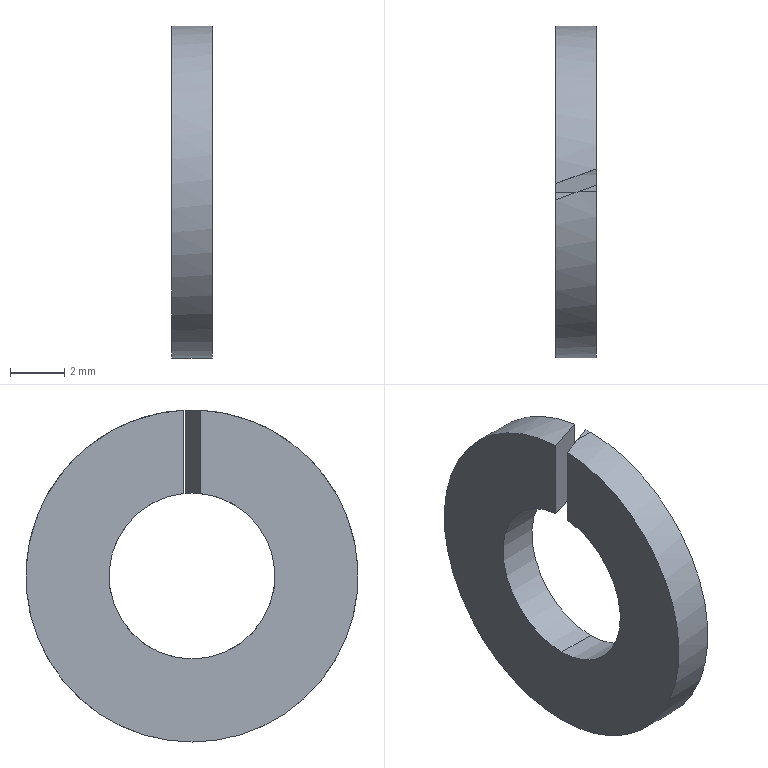Part | STEP file | 0217_302_SLW6 | 1 solid | 10 faces | box 1.5 x 12.2 x 12.2 mm | volume 128.756 mm3 | cylinder 6 | plane 4 | commonest cylinder face diameters 6.1 x3 12.2 x3
STEP:
#1=CARTESIAN_POINT('',(0.,0.,0.));
#2=DIRECTION('',(0.,0.,1.));
#3=DIRECTION('',(1.,0.,0.));
#4=AXIS2_PLACEMENT_3D('',#1,#2,#3);
#5=CARTESIAN_POINT('',(1.5,0.246,6.095));
#6=VERTEX_POINT('',#5);
#7=CARTESIAN_POINT('',(0.8242,0.,6.1));
#8=VERTEX_POINT('',#7);
#9=CARTESIAN_POINT('',(1.5,0.246,6.095));
#10=CARTESIAN_POINT('',(1.275,0.164,6.098));
#11=CARTESIAN_POINT('',(1.05,0.08201,6.1));
#12=CARTESIAN_POINT('',(0.8242,0.,6.1));
#13=(BOUNDED_CURVE()B_SPLINE_CURVE(3,(#9,#10,#11,#12),.UNSPECIFIED.,.F.,.F.)B_SPLINE_CURVE_WITH_KNOTS((4,4),(1.53,1.571),.PIECEWISE_BEZIER_KNOTS.)CURVE()GEOMETRIC_REPRESENTATION_ITEM()RATIONAL_B_SPLINE_CURVE((1.,0.9999,0.9999,1.))REPRESENTATION_ITEM(''));
#14=CARTESIAN_POINT('',(0.,0.,0.));
#15=DIRECTION('',(1.,0.,0.));
#16=DIRECTION('',(0.,0.,-1.));
#17=AXIS2_PLACEMENT_3D('',#14,#15,#16);
#18=CYLINDRICAL_SURFACE('',#17,6.1);
#19=CARTESIAN_POINT('',(3.101,1.5));
#20=CARTESIAN_POINT('',(3.102,1.49));
#21=CARTESIAN_POINT('',(3.103,1.469));
#22=CARTESIAN_POINT('',(3.105,1.439));
#23=CARTESIAN_POINT('',(3.107,1.408));
#24=CARTESIAN_POINT('',(3.109,1.377));
#25=CARTESIAN_POINT('',(3.11,1.346));
#26=CARTESIAN_POINT('',(3.112,1.316));
#27=CARTESIAN_POINT('',(3.114,1.285));
#28=CARTESIAN_POINT('',(3.116,1.254));
#29=CARTESIAN_POINT('',(3.118,1.224));
#30=CARTESIAN_POINT('',(3.12,1.193));
#31=CARTESIAN_POINT('',(3.121,1.162));
#32=CARTESIAN_POINT('',(3.123,1.131));
#33=CARTESIAN_POINT('',(3.125,1.101));
#34=CARTESIAN_POINT('',(3.127,1.07));
#35=CARTESIAN_POINT('',(3.129,1.039));
#36=CARTESIAN_POINT('',(3.131,1.009));
#37=CARTESIAN_POINT('',(3.132,0.9779));
#38=CARTESIAN_POINT('',(3.134,0.9471));
#39=CARTESIAN_POINT('',(3.136,0.9164));
#40=CARTESIAN_POINT('',(3.138,0.8857));
#41=CARTESIAN_POINT('',(3.14,0.855));
#42=CARTESIAN_POINT('',(3.141,0.8345));
#43=CARTESIAN_POINT('',(3.142,0.8242));
#44=B_SPLINE_CURVE_WITH_KNOTS('',3,(#19,#20,#21,#22,#23,#24,#25,#26,#27,#28,#29,#30,#31,#32,#33,#34,#35,#36,#37,#38,#39,#40,#41,#42,#43),.UNSPECIFIED.,.F.,.F.,(4,1,1,1,1,1,1,1,1,1,1,1,1,1,1,1,1,1,1,1,1,1,4),(1.53,1.532,1.534,1.536,1.538,1.54,1.541,1.543,1.545,1.547,1.549,1.551,1.552,1.554,1.556,1.558,1.56,1.562,1.563,1.565,1.567,1.569,1.571),.QUASI_UNIFORM_KNOTS.);
#45=(GEOMETRIC_REPRESENTATION_CONTEXT(2)PARAMETRIC_REPRESENTATION_CONTEXT()REPRESENTATION_CONTEXT('',''));
#46=DEFINITIONAL_REPRESENTATION('',(#44),#45);
#47=PCURVE('',#18,#46);
#48=CARTESIAN_POINT('',(1.5,0.246,0.));
#49=DIRECTION('',(0.342,-0.9397,0.));
#50=DIRECTION('',(0.9397,0.342,0.));
#51=AXIS2_PLACEMENT_3D('',#48,#49,#50);
#52=PLANE('',#51);
#53=CARTESIAN_POINT('',(0.,6.095));
#54=CARTESIAN_POINT('',(-0.2396,6.098));
#55=CARTESIAN_POINT('',(-0.4793,6.1));
#56=CARTESIAN_POINT('',(-0.7191,6.1));
#57=(BOUNDED_CURVE()B_SPLINE_CURVE(3,(#53,#54,#55,#56),.UNSPECIFIED.,.F.,.F.)B_SPLINE_CURVE_WITH_KNOTS((4,4),(1.53,1.571),.PIECEWISE_BEZIER_KNOTS.)CURVE()GEOMETRIC_REPRESENTATION_ITEM()RATIONAL_B_SPLINE_CURVE((1.,0.9999,0.9999,1.))REPRESENTATION_ITEM(''));
#58=(GEOMETRIC_REPRESENTATION_CONTEXT(2)PARAMETRIC_REPRESENTATION_CONTEXT()REPRESENTATION_CONTEXT('',''));
#59=DEFINITIONAL_REPRESENTATION('',(#57),#58);
#60=PCURVE('',#52,#59);
#61=SURFACE_CURVE('',#13,(#47,#60),.PCURVE_S1.);
#62=EDGE_CURVE('',#6,#8,#61,.T.);
#63=ORIENTED_EDGE('',*,*,#62,.T.);
#64=CARTESIAN_POINT('',(1.5,0.,6.1));
#65=VERTEX_POINT('',#64);
#66=CARTESIAN_POINT('',(0.,0.,6.1));
#67=DIRECTION('',(1.,0.,0.));
#68=VECTOR('',#67,1.);
#69=LINE('',#66,#68);
#70=CARTESIAN_POINT('',(3.142,0.));
#71=DIRECTION('',(0.,1.));
#72=VECTOR('',#71,1.);
#73=LINE('',#70,#72);
#74=(GEOMETRIC_REPRESENTATION_CONTEXT(2)PARAMETRIC_REPRESENTATION_CONTEXT()REPRESENTATION_CONTEXT('',''));
#75=DEFINITIONAL_REPRESENTATION('',(#73),#74);
#76=PCURVE('',#18,#75);
#77=CARTESIAN_POINT('',(0.,0.,0.));
#78=DIRECTION('',(1.,0.,0.));
#79=DIRECTION('',(0.,0.,-1.));
#80=AXIS2_PLACEMENT_3D('',#77,#78,#79);
#81=CYLINDRICAL_SURFACE('',#80,6.1);
#82=CARTESIAN_POINT('',(3.142,0.));
#83=DIRECTION('',(0.,1.));
#84=VECTOR('',#83,1.);
#85=LINE('',#82,#84);
#86=(GEOMETRIC_REPRESENTATION_CONTEXT(2)PARAMETRIC_REPRESENTATION_CONTEXT()REPRESENTATION_CONTEXT('',''));
#87=DEFINITIONAL_REPRESENTATION('',(#85),#86);
#88=PCURVE('',#81,#87);
#89=SURFACE_CURVE('',#69,(#76,#88),.PCURVE_S1.);
#90=EDGE_CURVE('',#8,#65,#89,.T.);
#91=ORIENTED_EDGE('',*,*,#90,.T.);
#92=CARTESIAN_POINT('',(1.5,0.,0.));
#93=DIRECTION('',(-1.,0.,0.));
#94=DIRECTION('',(0.,0.,-1.));
#95=AXIS2_PLACEMENT_3D('',#92,#93,#94);
#96=CIRCLE('',#95,6.1);
#97=CARTESIAN_POINT('',(6.283,1.5));
#98=DIRECTION('',(-1.,0.));
#99=VECTOR('',#98,1.);
#100=LINE('',#97,#99);
#101=(GEOMETRIC_REPRESENTATION_CONTEXT(2)PARAMETRIC_REPRESENTATION_CONTEXT()REPRESENTATION_CONTEXT('',''));
#102=DEFINITIONAL_REPRESENTATION('',(#100),#101);
#103=PCURVE('',#18,#102);
#104=CARTESIAN_POINT('',(1.5,0.,0.));
#105=DIRECTION('',(-1.,0.,0.));
#106=DIRECTION('',(0.,0.,1.));
#107=AXIS2_PLACEMENT_3D('',#104,#105,#106);
#108=PLANE('',#107);
#109=CARTESIAN_POINT('',(0.,0.));
#110=DIRECTION('',(-1.,0.));
#111=AXIS2_PLACEMENT_2D('',#109,#110);
#112=CIRCLE('',#111,6.1);
#113=(GEOMETRIC_REPRESENTATION_CONTEXT(2)PARAMETRIC_REPRESENTATION_CONTEXT()REPRESENTATION_CONTEXT('',''));
#114=DEFINITIONAL_REPRESENTATION('',(#112),#113);
#115=PCURVE('',#108,#114);
#116=SURFACE_CURVE('',#96,(#103,#115),.PCURVE_S1.);
#117=EDGE_CURVE('',#65,#6,#116,.T.);
#118=ORIENTED_EDGE('',*,*,#117,.T.);
#119=EDGE_LOOP('',(#63,#91,#118));
#120=FACE_BOUND('',#119,.T.);
#121=ADVANCED_FACE('',(#120),#18,.T.);
#122=ORIENTED_EDGE('',*,*,#90,.F.);
#123=CARTESIAN_POINT('',(0.,-0.3,6.093));
#124=VERTEX_POINT('',#123);
#125=CARTESIAN_POINT('',(0.8242,0.,6.1));
#126=CARTESIAN_POINT('',(0.5494,-0.1001,6.1));
#127=CARTESIAN_POINT('',(0.2746,-0.2001,6.098));
#128=CARTESIAN_POINT('',(0.,-0.3,6.093));
#129=(BOUNDED_CURVE()B_SPLINE_CURVE(3,(#125,#126,#127,#128),.UNSPECIFIED.,.F.,.F.)B_SPLINE_CURVE_WITH_KNOTS((4,4),(1.571,1.62),.PIECEWISE_BEZIER_KNOTS.)CURVE()GEOMETRIC_REPRESENTATION_ITEM()RATIONAL_B_SPLINE_CURVE((1.,0.9998,0.9998,1.))REPRESENTATION_ITEM(''));
#130=CARTESIAN_POINT('',(3.142,0.8242));
#131=CARTESIAN_POINT('',(3.142,0.8118));
#132=CARTESIAN_POINT('',(3.144,0.7868));
#133=CARTESIAN_POINT('',(3.146,0.7493));
#134=CARTESIAN_POINT('',(3.148,0.7118));
#135=CARTESIAN_POINT('',(3.151,0.6743));
#136=CARTESIAN_POINT('',(3.153,0.6369));
#137=CARTESIAN_POINT('',(3.155,0.5994));
#138=CARTESIAN_POINT('',(3.157,0.5619));
#139=CARTESIAN_POINT('',(3.159,0.5244));
#140=CARTESIAN_POINT('',(3.162,0.4869));
#141=CARTESIAN_POINT('',(3.164,0.4495));
#142=CARTESIAN_POINT('',(3.166,0.412));
#143=CARTESIAN_POINT('',(3.168,0.3745));
#144=CARTESIAN_POINT('',(3.171,0.3371));
#145=CARTESIAN_POINT('',(3.173,0.2996));
#146=CARTESIAN_POINT('',(3.175,0.2621));
#147=CARTESIAN_POINT('',(3.177,0.2247));
#148=CARTESIAN_POINT('',(3.18,0.1872));
#149=CARTESIAN_POINT('',(3.182,0.1498));
#150=CARTESIAN_POINT('',(3.184,0.1123));
#151=CARTESIAN_POINT('',(3.186,0.07487));
#152=CARTESIAN_POINT('',(3.189,0.03743));
#153=CARTESIAN_POINT('',(3.19,0.01248));
#154=CARTESIAN_POINT('',(3.191,0.));
#155=B_SPLINE_CURVE_WITH_KNOTS('',3,(#130,#131,#132,#133,#134,#135,#136,#137,#138,#139,#140,#141,#142,#143,#144,#145,#146,#147,#148,#149,#150,#151,#152,#153,#154),.UNSPECIFIED.,.F.,.F.,(4,1,1,1,1,1,1,1,1,1,1,1,1,1,1,1,1,1,1,1,1,1,4),(1.571,1.573,1.575,1.578,1.58,1.582,1.584,1.586,1.589,1.591,1.593,1.595,1.598,1.6,1.602,1.604,1.607,1.609,1.611,1.613,1.616,1.618,1.62),.QUASI_UNIFORM_KNOTS.);
#156=(GEOMETRIC_REPRESENTATION_CONTEXT(2)PARAMETRIC_REPRESENTATION_CONTEXT()REPRESENTATION_CONTEXT('',''));
#157=DEFINITIONAL_REPRESENTATION('',(#155),#156);
#158=PCURVE('',#81,#157);
#159=CARTESIAN_POINT('',(-0.7191,6.1));
#160=CARTESIAN_POINT('',(-1.012,6.1));
#161=CARTESIAN_POINT('',(-1.304,6.098));
#162=CARTESIAN_POINT('',(-1.596,6.093));
#163=(BOUNDED_CURVE()B_SPLINE_CURVE(3,(#159,#160,#161,#162),.UNSPECIFIED.,.F.,.F.)B_SPLINE_CURVE_WITH_KNOTS((4,4),(1.571,1.62),.PIECEWISE_BEZIER_KNOTS.)CURVE()GEOMETRIC_REPRESENTATION_ITEM()RATIONAL_B_SPLINE_CURVE((1.,0.9998,0.9998,1.))REPRESENTATION_ITEM(''));
#164=(GEOMETRIC_REPRESENTATION_CONTEXT(2)PARAMETRIC_REPRESENTATION_CONTEXT()REPRESENTATION_CONTEXT('',''));
#165=DEFINITIONAL_REPRESENTATION('',(#163),#164);
#166=PCURVE('',#52,#165);
#167=SURFACE_CURVE('',#129,(#158,#166),.PCURVE_S1.);
#168=EDGE_CURVE('',#8,#124,#167,.T.);
#169=ORIENTED_EDGE('',*,*,#168,.T.);
#170=CARTESIAN_POINT('',(0.,0.,-6.1));
#171=VERTEX_POINT('',#170);
#172=CARTESIAN_POINT('',(0.,0.,0.));
#173=DIRECTION('',(-1.,0.,0.));
#174=DIRECTION('',(0.,0.,-1.));
#175=AXIS2_PLACEMENT_3D('',#172,#173,#174);
#176=CIRCLE('',#175,6.1);
#177=CARTESIAN_POINT('',(6.283,0.));
#178=DIRECTION('',(-1.,0.));
#179=VECTOR('',#178,1.);
#180=LINE('',#177,#179);
#181=(GEOMETRIC_REPRESENTATION_CONTEXT(2)PARAMETRIC_REPRESENTATION_CONTEXT()REPRESENTATION_CONTEXT('',''));
#182=DEFINITIONAL_REPRESENTATION('',(#180),#181);
#183=PCURVE('',#81,#182);
#184=CARTESIAN_POINT('',(0.,0.,0.));
#185=DIRECTION('',(-1.,0.,0.));
#186=DIRECTION('',(0.,0.,1.));
#187=AXIS2_PLACEMENT_3D('',#184,#185,#186);
#188=PLANE('',#187);
#189=CARTESIAN_POINT('',(0.,0.));
#190=DIRECTION('',(-1.,0.));
#191=AXIS2_PLACEMENT_2D('',#189,#190);
#192=CIRCLE('',#191,6.1);
#193=(GEOMETRIC_REPRESENTATION_CONTEXT(2)PARAMETRIC_REPRESENTATION_CONTEXT()REPRESENTATION_CONTEXT('',''));
#194=DEFINITIONAL_REPRESENTATION('',(#192),#193);
#195=PCURVE('',#188,#194);
#196=SURFACE_CURVE('',#176,(#183,#195),.PCURVE_S1.);
#197=EDGE_CURVE('',#171,#124,#196,.T.);
#198=ORIENTED_EDGE('',*,*,#197,.F.);
#199=CARTESIAN_POINT('',(1.5,0.,-6.1));
#200=VERTEX_POINT('',#199);
#201=CARTESIAN_POINT('',(0.,0.,-6.1));
#202=DIRECTION('',(1.,0.,0.));
#203=VECTOR('',#202,1.);
#204=LINE('',#201,#203);
#205=CARTESIAN_POINT('',(6.283,0.));
#206=DIRECTION('',(0.,1.));
#207=VECTOR('',#206,1.);
#208=LINE('',#205,#207);
#209=(GEOMETRIC_REPRESENTATION_CONTEXT(2)PARAMETRIC_REPRESENTATION_CONTEXT()REPRESENTATION_CONTEXT('',''));
#210=DEFINITIONAL_REPRESENTATION('',(#208),#209);
#211=PCURVE('',#81,#210);
#212=CARTESIAN_POINT('',(0.,0.,0.));
#213=DIRECTION('',(1.,0.,0.));
#214=DIRECTION('',(0.,0.,-1.));
#215=AXIS2_PLACEMENT_3D('',#212,#213,#214);
#216=CYLINDRICAL_SURFACE('',#215,6.1);
#217=CARTESIAN_POINT('',(0.,0.));
#218=DIRECTION('',(0.,1.));
#219=VECTOR('',#218,1.);
#220=LINE('',#217,#219);
#221=(GEOMETRIC_REPRESENTATION_CONTEXT(2)PARAMETRIC_REPRESENTATION_CONTEXT()REPRESENTATION_CONTEXT('',''));
#222=DEFINITIONAL_REPRESENTATION('',(#220),#221);
#223=PCURVE('',#216,#222);
#224=SURFACE_CURVE('',#204,(#211,#223),.PCURVE_S1.);
#225=EDGE_CURVE('',#171,#200,#224,.T.);
#226=ORIENTED_EDGE('',*,*,#225,.T.);
#227=CARTESIAN_POINT('',(1.5,0.,0.));
#228=DIRECTION('',(-1.,0.,0.));
#229=DIRECTION('',(0.,0.,-1.));
#230=AXIS2_PLACEMENT_3D('',#227,#228,#229);
#231=CIRCLE('',#230,6.1);
#232=CARTESIAN_POINT('',(6.283,1.5));
#233=DIRECTION('',(-1.,0.));
#234=VECTOR('',#233,1.);
#235=LINE('',#232,#234);
#236=(GEOMETRIC_REPRESENTATION_CONTEXT(2)PARAMETRIC_REPRESENTATION_CONTEXT()REPRESENTATION_CONTEXT('',''));
#237=DEFINITIONAL_REPRESENTATION('',(#235),#236);
#238=PCURVE('',#81,#237);
#239=CARTESIAN_POINT('',(0.,0.));
#240=DIRECTION('',(-1.,0.));
#241=AXIS2_PLACEMENT_2D('',#239,#240);
#242=CIRCLE('',#241,6.1);
#243=(GEOMETRIC_REPRESENTATION_CONTEXT(2)PARAMETRIC_REPRESENTATION_CONTEXT()REPRESENTATION_CONTEXT('',''));
#244=DEFINITIONAL_REPRESENTATION('',(#242),#243);
#245=PCURVE('',#108,#244);
#246=SURFACE_CURVE('',#231,(#238,#245),.PCURVE_S1.);
#247=EDGE_CURVE('',#200,#65,#246,.T.);
#248=ORIENTED_EDGE('',*,*,#247,.T.);
#249=EDGE_LOOP('',(#122,#169,#198,#226,#248));
#250=FACE_BOUND('',#249,.T.);
#251=ADVANCED_FACE('',(#250),#81,.T.);
#252=CARTESIAN_POINT('',(0.,-0.3,3.035));
#253=VERTEX_POINT('',#252);
#254=CARTESIAN_POINT('',(0.,0.,-3.05));
#255=VERTEX_POINT('',#254);
#256=CARTESIAN_POINT('',(0.,0.,0.));
#257=DIRECTION('',(1.,0.,0.));
#258=DIRECTION('',(0.,0.,-1.));
#259=AXIS2_PLACEMENT_3D('',#256,#257,#258);
#260=CIRCLE('',#259,3.05);
#261=CARTESIAN_POINT('',(0.,0.,0.));
#262=DIRECTION('',(1.,0.,0.));
#263=DIRECTION('',(0.,0.,-1.));
#264=AXIS2_PLACEMENT_3D('',#261,#262,#263);
#265=CYLINDRICAL_SURFACE('',#264,3.05);
#266=CARTESIAN_POINT('',(0.,0.));
#267=DIRECTION('',(1.,0.));
#268=VECTOR('',#267,1.);
#269=LINE('',#266,#268);
#270=(GEOMETRIC_REPRESENTATION_CONTEXT(2)PARAMETRIC_REPRESENTATION_CONTEXT()REPRESENTATION_CONTEXT('',''));
#271=DEFINITIONAL_REPRESENTATION('',(#269),#270);
#272=PCURVE('',#265,#271);
#273=CARTESIAN_POINT('',(-3.05,0.));
#274=CARTESIAN_POINT('',(-3.05,5.283));
#275=CARTESIAN_POINT('',(1.525,2.641));
#276=CARTESIAN_POINT('',(6.1,0.));
#277=CARTESIAN_POINT('',(1.525,-2.641));
#278=CARTESIAN_POINT('',(-3.05,-5.283));
#279=CARTESIAN_POINT('',(-3.05,0.));
#280=(BOUNDED_CURVE()B_SPLINE_CURVE(2,(#273,#274,#275,#276,#277,#278,#279),.UNSPECIFIED.,.T.,.F.)B_SPLINE_CURVE_WITH_KNOTS((1,2,2,2,2,1),(-2.094,0.,2.094,4.189,6.283,8.378),.UNSPECIFIED.)CURVE()GEOMETRIC_REPRESENTATION_ITEM()RATIONAL_B_SPLINE_CURVE((1.,0.5,1.,0.5,1.,0.5,1.))REPRESENTATION_ITEM(''));
#281=(GEOMETRIC_REPRESENTATION_CONTEXT(2)PARAMETRIC_REPRESENTATION_CONTEXT()REPRESENTATION_CONTEXT('',''));
#282=DEFINITIONAL_REPRESENTATION('',(#280),#281);
#283=PCURVE('',#188,#282);
#284=SURFACE_CURVE('',#260,(#272,#283),.PCURVE_S1.);
#285=EDGE_CURVE('',#253,#255,#284,.T.);
#286=ORIENTED_EDGE('',*,*,#285,.T.);
#287=CARTESIAN_POINT('',(1.5,0.,-3.05));
#288=VERTEX_POINT('',#287);
#289=CARTESIAN_POINT('',(0.,0.,-3.05));
#290=DIRECTION('',(1.,0.,0.));
#291=VECTOR('',#290,1.);
#292=LINE('',#289,#291);
#293=CARTESIAN_POINT('',(6.283,0.));
#294=DIRECTION('',(0.,1.));
#295=VECTOR('',#294,1.);
#296=LINE('',#293,#295);
#297=(GEOMETRIC_REPRESENTATION_CONTEXT(2)PARAMETRIC_REPRESENTATION_CONTEXT()REPRESENTATION_CONTEXT('',''));
#298=DEFINITIONAL_REPRESENTATION('',(#296),#297);
#299=PCURVE('',#265,#298);
#300=CARTESIAN_POINT('',(0.,0.,0.));
#301=DIRECTION('',(1.,0.,0.));
#302=DIRECTION('',(0.,0.,-1.));
#303=AXIS2_PLACEMENT_3D('',#300,#301,#302);
#304=CYLINDRICAL_SURFACE('',#303,3.05);
#305=CARTESIAN_POINT('',(0.,0.));
#306=DIRECTION('',(0.,1.));
#307=VECTOR('',#306,1.);
#308=LINE('',#305,#307);
#309=(GEOMETRIC_REPRESENTATION_CONTEXT(2)PARAMETRIC_REPRESENTATION_CONTEXT()REPRESENTATION_CONTEXT('',''));
#310=DEFINITIONAL_REPRESENTATION('',(#308),#309);
#311=PCURVE('',#304,#310);
#312=SURFACE_CURVE('',#292,(#299,#311),.PCURVE_S1.);
#313=EDGE_CURVE('',#255,#288,#312,.T.);
#314=ORIENTED_EDGE('',*,*,#313,.T.);
#315=CARTESIAN_POINT('',(1.5,0.,3.05));
#316=VERTEX_POINT('',#315);
#317=CARTESIAN_POINT('',(1.5,0.,0.));
#318=DIRECTION('',(-1.,0.,0.));
#319=DIRECTION('',(0.,0.,-1.));
#320=AXIS2_PLACEMENT_3D('',#317,#318,#319);
#321=CIRCLE('',#320,3.05);
#322=CARTESIAN_POINT('',(6.283,1.5));
#323=DIRECTION('',(-1.,0.));
#324=VECTOR('',#323,1.);
#325=LINE('',#322,#324);
#326=(GEOMETRIC_REPRESENTATION_CONTEXT(2)PARAMETRIC_REPRESENTATION_CONTEXT()REPRESENTATION_CONTEXT('',''));
#327=DEFINITIONAL_REPRESENTATION('',(#325),#326);
#328=PCURVE('',#265,#327);
#329=CARTESIAN_POINT('',(0.,0.));
#330=DIRECTION('',(-1.,0.));
#331=AXIS2_PLACEMENT_2D('',#329,#330);
#332=CIRCLE('',#331,3.05);
#333=(GEOMETRIC_REPRESENTATION_CONTEXT(2)PARAMETRIC_REPRESENTATION_CONTEXT()REPRESENTATION_CONTEXT('',''));
#334=DEFINITIONAL_REPRESENTATION('',(#332),#333);
#335=PCURVE('',#108,#334);
#336=SURFACE_CURVE('',#321,(#328,#335),.PCURVE_S1.);
#337=EDGE_CURVE('',#288,#316,#336,.T.);
#338=ORIENTED_EDGE('',*,*,#337,.T.);
#339=CARTESIAN_POINT('',(0.8242,0.,3.05));
#340=VERTEX_POINT('',#339);
#341=CARTESIAN_POINT('',(0.,0.,3.05));
#342=DIRECTION('',(1.,0.,0.));
#343=VECTOR('',#342,1.);
#344=LINE('',#341,#343);
#345=CARTESIAN_POINT('',(3.142,0.));
#346=DIRECTION('',(0.,1.));
#347=VECTOR('',#346,1.);
#348=LINE('',#345,#347);
#349=(GEOMETRIC_REPRESENTATION_CONTEXT(2)PARAMETRIC_REPRESENTATION_CONTEXT()REPRESENTATION_CONTEXT('',''));
#350=DEFINITIONAL_REPRESENTATION('',(#348),#349);
#351=PCURVE('',#265,#350);
#352=CARTESIAN_POINT('',(0.,0.,0.));
#353=DIRECTION('',(1.,0.,0.));
#354=DIRECTION('',(0.,0.,-1.));
#355=AXIS2_PLACEMENT_3D('',#352,#353,#354);
#356=CYLINDRICAL_SURFACE('',#355,3.05);
#357=CARTESIAN_POINT('',(3.142,0.));
#358=DIRECTION('',(0.,1.));
#359=VECTOR('',#358,1.);
#360=LINE('',#357,#359);
#361=(GEOMETRIC_REPRESENTATION_CONTEXT(2)PARAMETRIC_REPRESENTATION_CONTEXT()REPRESENTATION_CONTEXT('',''));
#362=DEFINITIONAL_REPRESENTATION('',(#360),#361);
#363=PCURVE('',#356,#362);
#364=SURFACE_CURVE('',#344,(#351,#363),.PCURVE_S1.);
#365=EDGE_CURVE('',#340,#316,#364,.T.);
#366=ORIENTED_EDGE('',*,*,#365,.F.);
#367=CARTESIAN_POINT('',(0.8242,0.,3.05));
#368=CARTESIAN_POINT('',(0.5489,-0.1002,3.05));
#369=CARTESIAN_POINT('',(0.274,-0.2003,3.045));
#370=CARTESIAN_POINT('',(0.,-0.3,3.035));
#371=(BOUNDED_CURVE()B_SPLINE_CURVE(3,(#367,#368,#369,#370),.UNSPECIFIED.,.F.,.F.)B_SPLINE_CURVE_WITH_KNOTS((4,4),(1.571,1.669),.PIECEWISE_BEZIER_KNOTS.)CURVE()GEOMETRIC_REPRESENTATION_ITEM()RATIONAL_B_SPLINE_CURVE((1.,0.9992,0.9992,1.))REPRESENTATION_ITEM(''));
#372=CARTESIAN_POINT('',(3.142,0.8242));
#373=CARTESIAN_POINT('',(3.143,0.8117));
#374=CARTESIAN_POINT('',(3.146,0.7867));
#375=CARTESIAN_POINT('',(3.151,0.7492));
#376=CARTESIAN_POINT('',(3.155,0.7117));
#377=CARTESIAN_POINT('',(3.16,0.6742));
#378=CARTESIAN_POINT('',(3.164,0.6367));
#379=CARTESIAN_POINT('',(3.168,0.5991));
#380=CARTESIAN_POINT('',(3.173,0.5616));
#381=CARTESIAN_POINT('',(3.177,0.5241));
#382=CARTESIAN_POINT('',(3.182,0.4866));
#383=CARTESIAN_POINT('',(3.186,0.4491));
#384=CARTESIAN_POINT('',(3.191,0.4116));
#385=CARTESIAN_POINT('',(3.195,0.3741));
#386=CARTESIAN_POINT('',(3.2,0.3367));
#387=CARTESIAN_POINT('',(3.204,0.2992));
#388=CARTESIAN_POINT('',(3.209,0.2617));
#389=CARTESIAN_POINT('',(3.213,0.2243));
#390=CARTESIAN_POINT('',(3.218,0.1869));
#391=CARTESIAN_POINT('',(3.222,0.1495));
#392=CARTESIAN_POINT('',(3.227,0.1121));
#393=CARTESIAN_POINT('',(3.231,0.0747));
#394=CARTESIAN_POINT('',(3.236,0.03734));
#395=CARTESIAN_POINT('',(3.239,0.01244));
#396=CARTESIAN_POINT('',(3.24,0.));
#397=B_SPLINE_CURVE_WITH_KNOTS('',3,(#372,#373,#374,#375,#376,#377,#378,#379,#380,#381,#382,#383,#384,#385,#386,#387,#388,#389,#390,#391,#392,#393,#394,#395,#396),.UNSPECIFIED.,.F.,.F.,(4,1,1,1,1,1,1,1,1,1,1,1,1,1,1,1,1,1,1,1,1,1,4),(1.571,1.575,1.58,1.584,1.589,1.593,1.598,1.602,1.607,1.611,1.616,1.62,1.625,1.629,1.633,1.638,1.642,1.647,1.651,1.656,1.66,1.665,1.669),.QUASI_UNIFORM_KNOTS.);
#398=(GEOMETRIC_REPRESENTATION_CONTEXT(2)PARAMETRIC_REPRESENTATION_CONTEXT()REPRESENTATION_CONTEXT('',''));
#399=DEFINITIONAL_REPRESENTATION('',(#397),#398);
#400=PCURVE('',#265,#399);
#401=CARTESIAN_POINT('',(-0.7191,3.05));
#402=CARTESIAN_POINT('',(-1.012,3.05));
#403=CARTESIAN_POINT('',(-1.305,3.045));
#404=CARTESIAN_POINT('',(-1.596,3.035));
#405=(BOUNDED_CURVE()B_SPLINE_CURVE(3,(#401,#402,#403,#404),.UNSPECIFIED.,.F.,.F.)B_SPLINE_CURVE_WITH_KNOTS((4,4),(1.571,1.669),.PIECEWISE_BEZIER_KNOTS.)CURVE()GEOMETRIC_REPRESENTATION_ITEM()RATIONAL_B_SPLINE_CURVE((1.,0.9992,0.9992,1.))REPRESENTATION_ITEM(''));
#406=(GEOMETRIC_REPRESENTATION_CONTEXT(2)PARAMETRIC_REPRESENTATION_CONTEXT()REPRESENTATION_CONTEXT('',''));
#407=DEFINITIONAL_REPRESENTATION('',(#405),#406);
#408=PCURVE('',#52,#407);
#409=SURFACE_CURVE('',#371,(#400,#408),.PCURVE_S1.);
#410=EDGE_CURVE('',#340,#253,#409,.T.);
#411=ORIENTED_EDGE('',*,*,#410,.T.);
#412=EDGE_LOOP('',(#286,#314,#338,#366,#411));
#413=FACE_BOUND('',#412,.F.);
#414=ADVANCED_FACE('',(#413),#265,.F.);
#415=CARTESIAN_POINT('',(1.5,0.846,2.93));
#416=VERTEX_POINT('',#415);
#417=CARTESIAN_POINT('',(0.,0.3,3.035));
#418=VERTEX_POINT('',#417);
#419=CARTESIAN_POINT('',(1.5,0.846,2.93));
#420=CARTESIAN_POINT('',(1.009,0.6674,2.982));
#421=CARTESIAN_POINT('',(0.5081,0.4849,3.017));
#422=CARTESIAN_POINT('',(0.,0.3,3.035));
#423=(BOUNDED_CURVE()B_SPLINE_CURVE(3,(#419,#420,#421,#422),.UNSPECIFIED.,.F.,.F.)B_SPLINE_CURVE_WITH_KNOTS((4,4),(1.29,1.472),.PIECEWISE_BEZIER_KNOTS.)CURVE()GEOMETRIC_REPRESENTATION_ITEM()RATIONAL_B_SPLINE_CURVE((1.,0.9972,0.9972,1.))REPRESENTATION_ITEM(''));
#424=CARTESIAN_POINT('',(2.861,1.5));
#425=CARTESIAN_POINT('',(2.863,1.478));
#426=CARTESIAN_POINT('',(2.869,1.433));
#427=CARTESIAN_POINT('',(2.877,1.366));
#428=CARTESIAN_POINT('',(2.885,1.299));
#429=CARTESIAN_POINT('',(2.894,1.232));
#430=CARTESIAN_POINT('',(2.902,1.164));
#431=CARTESIAN_POINT('',(2.91,1.097));
#432=CARTESIAN_POINT('',(2.919,1.029));
#433=CARTESIAN_POINT('',(2.927,0.9611));
#434=CARTESIAN_POINT('',(2.935,0.893));
#435=CARTESIAN_POINT('',(2.944,0.8249));
#436=CARTESIAN_POINT('',(2.952,0.7566));
#437=CARTESIAN_POINT('',(2.96,0.6882));
#438=CARTESIAN_POINT('',(2.968,0.6197));
#439=CARTESIAN_POINT('',(2.977,0.5512));
#440=CARTESIAN_POINT('',(2.985,0.4825));
#441=CARTESIAN_POINT('',(2.993,0.4138));
#442=CARTESIAN_POINT('',(3.002,0.3449));
#443=CARTESIAN_POINT('',(3.01,0.2761));
#444=CARTESIAN_POINT('',(3.018,0.2071));
#445=CARTESIAN_POINT('',(3.026,0.1381));
#446=CARTESIAN_POINT('',(3.035,0.06908));
#447=CARTESIAN_POINT('',(3.04,0.02303));
#448=CARTESIAN_POINT('',(3.043,0.));
#449=B_SPLINE_CURVE_WITH_KNOTS('',3,(#424,#425,#426,#427,#428,#429,#430,#431,#432,#433,#434,#435,#436,#437,#438,#439,#440,#441,#442,#443,#444,#445,#446,#447,#448),.UNSPECIFIED.,.F.,.F.,(4,1,1,1,1,1,1,1,1,1,1,1,1,1,1,1,1,1,1,1,1,1,4),(1.29,1.298,1.306,1.315,1.323,1.331,1.34,1.348,1.356,1.364,1.373,1.381,1.389,1.398,1.406,1.414,1.422,1.431,1.439,1.447,1.456,1.464,1.472),.QUASI_UNIFORM_KNOTS.);
#450=(GEOMETRIC_REPRESENTATION_CONTEXT(2)PARAMETRIC_REPRESENTATION_CONTEXT()REPRESENTATION_CONTEXT('',''));
#451=DEFINITIONAL_REPRESENTATION('',(#449),#450);
#452=PCURVE('',#304,#451);
#453=CARTESIAN_POINT('',(0.,0.3,0.));
#454=DIRECTION('',(-0.342,0.9397,0.));
#455=DIRECTION('',(-0.9397,-0.342,0.));
#456=AXIS2_PLACEMENT_3D('',#453,#454,#455);
#457=PLANE('',#456);
#458=CARTESIAN_POINT('',(-1.596,2.93));
#459=CARTESIAN_POINT('',(-1.074,2.982));
#460=CARTESIAN_POINT('',(-0.5407,3.017));
#461=CARTESIAN_POINT('',(0.,3.035));
#462=(BOUNDED_CURVE()B_SPLINE_CURVE(3,(#458,#459,#460,#461),.UNSPECIFIED.,.F.,.F.)B_SPLINE_CURVE_WITH_KNOTS((4,4),(1.29,1.472),.PIECEWISE_BEZIER_KNOTS.)CURVE()GEOMETRIC_REPRESENTATION_ITEM()RATIONAL_B_SPLINE_CURVE((1.,0.9972,0.9972,1.))REPRESENTATION_ITEM(''));
#463=(GEOMETRIC_REPRESENTATION_CONTEXT(2)PARAMETRIC_REPRESENTATION_CONTEXT()REPRESENTATION_CONTEXT('',''));
#464=DEFINITIONAL_REPRESENTATION('',(#462),#463);
#465=PCURVE('',#457,#464);
#466=SURFACE_CURVE('',#423,(#452,#465),.PCURVE_S1.);
#467=EDGE_CURVE('',#416,#418,#466,.T.);
#468=ORIENTED_EDGE('',*,*,#467,.F.);
#469=CARTESIAN_POINT('',(1.5,0.,0.));
#470=DIRECTION('',(-1.,0.,0.));
#471=DIRECTION('',(0.,0.,-1.));
#472=AXIS2_PLACEMENT_3D('',#469,#470,#471);
#473=CIRCLE('',#472,3.05);
#474=CARTESIAN_POINT('',(6.283,1.5));
#475=DIRECTION('',(-1.,0.));
#476=VECTOR('',#475,1.);
#477=LINE('',#474,#476);
#478=(GEOMETRIC_REPRESENTATION_CONTEXT(2)PARAMETRIC_REPRESENTATION_CONTEXT()REPRESENTATION_CONTEXT('',''));
#479=DEFINITIONAL_REPRESENTATION('',(#477),#478);
#480=PCURVE('',#304,#479);
#481=CARTESIAN_POINT('',(0.,0.));
#482=DIRECTION('',(-1.,0.));
#483=AXIS2_PLACEMENT_2D('',#481,#482);
#484=CIRCLE('',#483,3.05);
#485=(GEOMETRIC_REPRESENTATION_CONTEXT(2)PARAMETRIC_REPRESENTATION_CONTEXT()REPRESENTATION_CONTEXT('',''));
#486=DEFINITIONAL_REPRESENTATION('',(#484),#485);
#487=PCURVE('',#108,#486);
#488=SURFACE_CURVE('',#473,(#480,#487),.PCURVE_S1.);
#489=EDGE_CURVE('',#416,#288,#488,.T.);
#490=ORIENTED_EDGE('',*,*,#489,.T.);
#491=ORIENTED_EDGE('',*,*,#313,.F.);
#492=CARTESIAN_POINT('',(0.,0.,0.));
#493=DIRECTION('',(1.,0.,0.));
#494=DIRECTION('',(0.,0.,-1.));
#495=AXIS2_PLACEMENT_3D('',#492,#493,#494);
#496=CIRCLE('',#495,3.05);
#497=CARTESIAN_POINT('',(0.,0.));
#498=DIRECTION('',(1.,0.));
#499=VECTOR('',#498,1.);
#500=LINE('',#497,#499);
#501=(GEOMETRIC_REPRESENTATION_CONTEXT(2)PARAMETRIC_REPRESENTATION_CONTEXT()REPRESENTATION_CONTEXT('',''));
#502=DEFINITIONAL_REPRESENTATION('',(#500),#501);
#503=PCURVE('',#304,#502);
#504=CARTESIAN_POINT('',(-3.05,0.));
#505=CARTESIAN_POINT('',(-3.05,5.283));
#506=CARTESIAN_POINT('',(1.525,2.641));
#507=CARTESIAN_POINT('',(6.1,0.));
#508=CARTESIAN_POINT('',(1.525,-2.641));
#509=CARTESIAN_POINT('',(-3.05,-5.283));
#510=CARTESIAN_POINT('',(-3.05,0.));
#511=(BOUNDED_CURVE()B_SPLINE_CURVE(2,(#504,#505,#506,#507,#508,#509,#510),.UNSPECIFIED.,.T.,.F.)B_SPLINE_CURVE_WITH_KNOTS((1,2,2,2,2,1),(-2.094,0.,2.094,4.189,6.283,8.378),.UNSPECIFIED.)CURVE()GEOMETRIC_REPRESENTATION_ITEM()RATIONAL_B_SPLINE_CURVE((1.,0.5,1.,0.5,1.,0.5,1.))REPRESENTATION_ITEM(''));
#512=(GEOMETRIC_REPRESENTATION_CONTEXT(2)PARAMETRIC_REPRESENTATION_CONTEXT()REPRESENTATION_CONTEXT('',''));
#513=DEFINITIONAL_REPRESENTATION('',(#511),#512);
#514=PCURVE('',#188,#513);
#515=SURFACE_CURVE('',#496,(#503,#514),.PCURVE_S1.);
#516=EDGE_CURVE('',#255,#418,#515,.T.);
#517=ORIENTED_EDGE('',*,*,#516,.T.);
#518=EDGE_LOOP('',(#468,#490,#491,#517));
#519=FACE_BOUND('',#518,.F.);
#520=ADVANCED_FACE('',(#519),#304,.F.);
#521=CARTESIAN_POINT('',(0.,0.3,6.093));
#522=VERTEX_POINT('',#521);
#523=CARTESIAN_POINT('',(0.,0.3,0.));
#524=DIRECTION('',(0.,0.,1.));
#525=VECTOR('',#524,1.);
#526=LINE('',#523,#525);
#527=CARTESIAN_POINT('',(0.,0.3));
#528=DIRECTION('',(1.,0.));
#529=VECTOR('',#528,1.);
#530=LINE('',#527,#529);
#531=(GEOMETRIC_REPRESENTATION_CONTEXT(2)PARAMETRIC_REPRESENTATION_CONTEXT()REPRESENTATION_CONTEXT('',''));
#532=DEFINITIONAL_REPRESENTATION('',(#530),#531);
#533=PCURVE('',#188,#532);
#534=CARTESIAN_POINT('',(0.,0.));
#535=DIRECTION('',(0.,1.));
#536=VECTOR('',#535,1.);
#537=LINE('',#534,#536);
#538=(GEOMETRIC_REPRESENTATION_CONTEXT(2)PARAMETRIC_REPRESENTATION_CONTEXT()REPRESENTATION_CONTEXT('',''));
#539=DEFINITIONAL_REPRESENTATION('',(#537),#538);
#540=PCURVE('',#457,#539);
#541=SURFACE_CURVE('',#526,(#533,#540),.PCURVE_S1.);
#542=EDGE_CURVE('',#418,#522,#541,.T.);
#543=ORIENTED_EDGE('',*,*,#542,.T.);
#544=CARTESIAN_POINT('',(0.,0.,0.));
#545=DIRECTION('',(-1.,0.,0.));
#546=DIRECTION('',(0.,0.,-1.));
#547=AXIS2_PLACEMENT_3D('',#544,#545,#546);
#548=CIRCLE('',#547,6.1);
#549=CARTESIAN_POINT('',(0.,0.));
#550=DIRECTION('',(-1.,0.));
#551=AXIS2_PLACEMENT_2D('',#549,#550);
#552=CIRCLE('',#551,6.1);
#553=(GEOMETRIC_REPRESENTATION_CONTEXT(2)PARAMETRIC_REPRESENTATION_CONTEXT()REPRESENTATION_CONTEXT('',''));
#554=DEFINITIONAL_REPRESENTATION('',(#552),#553);
#555=PCURVE('',#188,#554);
#556=CARTESIAN_POINT('',(6.283,0.));
#557=DIRECTION('',(-1.,0.));
#558=VECTOR('',#557,1.);
#559=LINE('',#556,#558);
#560=(GEOMETRIC_REPRESENTATION_CONTEXT(2)PARAMETRIC_REPRESENTATION_CONTEXT()REPRESENTATION_CONTEXT('',''));
#561=DEFINITIONAL_REPRESENTATION('',(#559),#560);
#562=PCURVE('',#216,#561);
#563=SURFACE_CURVE('',#548,(#555,#562),.PCURVE_S1.);
#564=EDGE_CURVE('',#522,#171,#563,.T.);
#565=ORIENTED_EDGE('',*,*,#564,.T.);
#566=ORIENTED_EDGE('',*,*,#197,.T.);
#567=CARTESIAN_POINT('',(0.,-0.3,0.));
#568=DIRECTION('',(0.,0.,-1.));
#569=VECTOR('',#568,1.);
#570=LINE('',#567,#569);
#571=CARTESIAN_POINT('',(0.,-0.3));
#572=DIRECTION('',(-1.,0.));
#573=VECTOR('',#572,1.);
#574=LINE('',#571,#573);
#575=(GEOMETRIC_REPRESENTATION_CONTEXT(2)PARAMETRIC_REPRESENTATION_CONTEXT()REPRESENTATION_CONTEXT('',''));
#576=DEFINITIONAL_REPRESENTATION('',(#574),#575);
#577=PCURVE('',#188,#576);
#578=CARTESIAN_POINT('',(-1.596,0.));
#579=DIRECTION('',(0.,-1.));
#580=VECTOR('',#579,1.);
#581=LINE('',#578,#580);
#582=(GEOMETRIC_REPRESENTATION_CONTEXT(2)PARAMETRIC_REPRESENTATION_CONTEXT()REPRESENTATION_CONTEXT('',''));
#583=DEFINITIONAL_REPRESENTATION('',(#581),#582);
#584=PCURVE('',#52,#583);
#585=SURFACE_CURVE('',#570,(#577,#584),.PCURVE_S1.);
#586=EDGE_CURVE('',#124,#253,#585,.T.);
#587=ORIENTED_EDGE('',*,*,#586,.T.);
#588=ORIENTED_EDGE('',*,*,#285,.T.);
#589=ORIENTED_EDGE('',*,*,#516,.T.);
#590=EDGE_LOOP('',(#543,#565,#566,#587,#588,#589));
#591=FACE_BOUND('',#590,.T.);
#592=ADVANCED_FACE('',(#591),#188,.T.);
#593=ORIENTED_EDGE('',*,*,#225,.F.);
#594=ORIENTED_EDGE('',*,*,#564,.F.);
#595=CARTESIAN_POINT('',(1.5,0.846,6.041));
#596=VERTEX_POINT('',#595);
#597=CARTESIAN_POINT('',(0.,0.3,6.093));
#598=CARTESIAN_POINT('',(0.502,0.4827,6.084));
#599=CARTESIAN_POINT('',(1.002,0.6648,6.066));
#600=CARTESIAN_POINT('',(1.5,0.846,6.041));
#601=(BOUNDED_CURVE()B_SPLINE_CURVE(3,(#597,#598,#599,#600),.UNSPECIFIED.,.F.,.F.)B_SPLINE_CURVE_WITH_KNOTS((4,4),(4.762,4.852),.PIECEWISE_BEZIER_KNOTS.)CURVE()GEOMETRIC_REPRESENTATION_ITEM()RATIONAL_B_SPLINE_CURVE((1.,0.9993,0.9993,1.))REPRESENTATION_ITEM(''));
#602=CARTESIAN_POINT('',(3.092,0.));
#603=CARTESIAN_POINT('',(3.091,0.0228));
#604=CARTESIAN_POINT('',(3.088,0.0684));
#605=CARTESIAN_POINT('',(3.084,0.1368));
#606=CARTESIAN_POINT('',(3.08,0.2052));
#607=CARTESIAN_POINT('',(3.076,0.2735));
#608=CARTESIAN_POINT('',(3.072,0.3419));
#609=CARTESIAN_POINT('',(3.068,0.4102));
#610=CARTESIAN_POINT('',(3.064,0.4785));
#611=CARTESIAN_POINT('',(3.06,0.5468));
#612=CARTESIAN_POINT('',(3.056,0.6151));
#613=CARTESIAN_POINT('',(3.052,0.6834));
#614=CARTESIAN_POINT('',(3.047,0.7516));
#615=CARTESIAN_POINT('',(3.043,0.8198));
#616=CARTESIAN_POINT('',(3.039,0.888));
#617=CARTESIAN_POINT('',(3.035,0.9561));
#618=CARTESIAN_POINT('',(3.031,1.024));
#619=CARTESIAN_POINT('',(3.027,1.092));
#620=CARTESIAN_POINT('',(3.023,1.16));
#621=CARTESIAN_POINT('',(3.019,1.228));
#622=CARTESIAN_POINT('',(3.015,1.296));
#623=CARTESIAN_POINT('',(3.011,1.364));
#624=CARTESIAN_POINT('',(3.007,1.432));
#625=CARTESIAN_POINT('',(3.004,1.477));
#626=CARTESIAN_POINT('',(3.002,1.5));
#627=B_SPLINE_CURVE_WITH_KNOTS('',3,(#602,#603,#604,#605,#606,#607,#608,#609,#610,#611,#612,#613,#614,#615,#616,#617,#618,#619,#620,#621,#622,#623,#624,#625,#626),.UNSPECIFIED.,.F.,.F.,(4,1,1,1,1,1,1,1,1,1,1,1,1,1,1,1,1,1,1,1,1,1,4),(4.762,4.766,4.77,4.774,4.778,4.782,4.786,4.79,4.794,4.798,4.802,4.807,4.811,4.815,4.819,4.823,4.827,4.831,4.835,4.839,4.843,4.847,4.852),.QUASI_UNIFORM_KNOTS.);
#628=(GEOMETRIC_REPRESENTATION_CONTEXT(2)PARAMETRIC_REPRESENTATION_CONTEXT()REPRESENTATION_CONTEXT('',''));
#629=DEFINITIONAL_REPRESENTATION('',(#627),#628);
#630=PCURVE('',#216,#629);
#631=CARTESIAN_POINT('',(0.,6.093));
#632=CARTESIAN_POINT('',(-0.5342,6.084));
#633=CARTESIAN_POINT('',(-1.067,6.066));
#634=CARTESIAN_POINT('',(-1.596,6.041));
#635=(BOUNDED_CURVE()B_SPLINE_CURVE(3,(#631,#632,#633,#634),.UNSPECIFIED.,.F.,.F.)B_SPLINE_CURVE_WITH_KNOTS((4,4),(4.762,4.852),.PIECEWISE_BEZIER_KNOTS.)CURVE()GEOMETRIC_REPRESENTATION_ITEM()RATIONAL_B_SPLINE_CURVE((1.,0.9993,0.9993,1.))REPRESENTATION_ITEM(''));
#636=(GEOMETRIC_REPRESENTATION_CONTEXT(2)PARAMETRIC_REPRESENTATION_CONTEXT()REPRESENTATION_CONTEXT('',''));
#637=DEFINITIONAL_REPRESENTATION('',(#635),#636);
#638=PCURVE('',#457,#637);
#639=SURFACE_CURVE('',#601,(#630,#638),.PCURVE_S1.);
#640=EDGE_CURVE('',#522,#596,#639,.T.);
#641=ORIENTED_EDGE('',*,*,#640,.T.);
#642=CARTESIAN_POINT('',(1.5,0.,0.));
#643=DIRECTION('',(-1.,0.,0.));
#644=DIRECTION('',(0.,0.,-1.));
#645=AXIS2_PLACEMENT_3D('',#642,#643,#644);
#646=CIRCLE('',#645,6.1);
#647=CARTESIAN_POINT('',(6.283,1.5));
#648=DIRECTION('',(-1.,0.));
#649=VECTOR('',#648,1.);
#650=LINE('',#647,#649);
#651=(GEOMETRIC_REPRESENTATION_CONTEXT(2)PARAMETRIC_REPRESENTATION_CONTEXT()REPRESENTATION_CONTEXT('',''));
#652=DEFINITIONAL_REPRESENTATION('',(#650),#651);
#653=PCURVE('',#216,#652);
#654=CARTESIAN_POINT('',(0.,0.));
#655=DIRECTION('',(-1.,0.));
#656=AXIS2_PLACEMENT_2D('',#654,#655);
#657=CIRCLE('',#656,6.1);
#658=(GEOMETRIC_REPRESENTATION_CONTEXT(2)PARAMETRIC_REPRESENTATION_CONTEXT()REPRESENTATION_CONTEXT('',''));
#659=DEFINITIONAL_REPRESENTATION('',(#657),#658);
#660=PCURVE('',#108,#659);
#661=SURFACE_CURVE('',#646,(#653,#660),.PCURVE_S1.);
#662=EDGE_CURVE('',#596,#200,#661,.T.);
#663=ORIENTED_EDGE('',*,*,#662,.T.);
#664=EDGE_LOOP('',(#593,#594,#641,#663));
#665=FACE_BOUND('',#664,.T.);
#666=ADVANCED_FACE('',(#665),#216,.T.);
#667=CARTESIAN_POINT('',(1.5,0.846,0.));
#668=DIRECTION('',(0.,0.,-1.));
#669=VECTOR('',#668,1.);
#670=LINE('',#667,#669);
#671=CARTESIAN_POINT('',(-1.596,0.));
#672=DIRECTION('',(0.,-1.));
#673=VECTOR('',#672,1.);
#674=LINE('',#671,#673);
#675=(GEOMETRIC_REPRESENTATION_CONTEXT(2)PARAMETRIC_REPRESENTATION_CONTEXT()REPRESENTATION_CONTEXT('',''));
#676=DEFINITIONAL_REPRESENTATION('',(#674),#675);
#677=PCURVE('',#457,#676);
#678=CARTESIAN_POINT('',(0.,0.846));
#679=DIRECTION('',(-1.,0.));
#680=VECTOR('',#679,1.);
#681=LINE('',#678,#680);
#682=(GEOMETRIC_REPRESENTATION_CONTEXT(2)PARAMETRIC_REPRESENTATION_CONTEXT()REPRESENTATION_CONTEXT('',''));
#683=DEFINITIONAL_REPRESENTATION('',(#681),#682);
#684=PCURVE('',#108,#683);
#685=SURFACE_CURVE('',#670,(#677,#684),.PCURVE_S1.);
#686=EDGE_CURVE('',#596,#416,#685,.T.);
#687=ORIENTED_EDGE('',*,*,#686,.F.);
#688=ORIENTED_EDGE('',*,*,#640,.F.);
#689=ORIENTED_EDGE('',*,*,#542,.F.);
#690=ORIENTED_EDGE('',*,*,#467,.F.);
#691=EDGE_LOOP('',(#687,#688,#689,#690));
#692=FACE_BOUND('',#691,.T.);
#693=ADVANCED_FACE('',(#692),#457,.F.);
#694=CARTESIAN_POINT('',(1.5,0.246,3.04));
#695=VERTEX_POINT('',#694);
#696=CARTESIAN_POINT('',(1.5,0.,0.));
#697=DIRECTION('',(-1.,0.,0.));
#698=DIRECTION('',(0.,0.,-1.));
#699=AXIS2_PLACEMENT_3D('',#696,#697,#698);
#700=CIRCLE('',#699,3.05);
#701=CARTESIAN_POINT('',(6.283,1.5));
#702=DIRECTION('',(-1.,0.));
#703=VECTOR('',#702,1.);
#704=LINE('',#701,#703);
#705=(GEOMETRIC_REPRESENTATION_CONTEXT(2)PARAMETRIC_REPRESENTATION_CONTEXT()REPRESENTATION_CONTEXT('',''));
#706=DEFINITIONAL_REPRESENTATION('',(#704),#705);
#707=PCURVE('',#356,#706);
#708=CARTESIAN_POINT('',(0.,0.));
#709=DIRECTION('',(-1.,0.));
#710=AXIS2_PLACEMENT_2D('',#708,#709);
#711=CIRCLE('',#710,3.05);
#712=(GEOMETRIC_REPRESENTATION_CONTEXT(2)PARAMETRIC_REPRESENTATION_CONTEXT()REPRESENTATION_CONTEXT('',''));
#713=DEFINITIONAL_REPRESENTATION('',(#711),#712);
#714=PCURVE('',#108,#713);
#715=SURFACE_CURVE('',#700,(#707,#714),.PCURVE_S1.);
#716=EDGE_CURVE('',#316,#695,#715,.T.);
#717=ORIENTED_EDGE('',*,*,#716,.T.);
#718=CARTESIAN_POINT('',(1.5,0.246,3.04));
#719=CARTESIAN_POINT('',(1.275,0.1641,3.047));
#720=CARTESIAN_POINT('',(1.05,0.0821,3.05));
#721=CARTESIAN_POINT('',(0.8242,0.,3.05));
#722=(BOUNDED_CURVE()B_SPLINE_CURVE(3,(#718,#719,#720,#721),.UNSPECIFIED.,.F.,.F.)B_SPLINE_CURVE_WITH_KNOTS((4,4),(1.49,1.571),.PIECEWISE_BEZIER_KNOTS.)CURVE()GEOMETRIC_REPRESENTATION_ITEM()RATIONAL_B_SPLINE_CURVE((1.,0.9995,0.9995,1.))REPRESENTATION_ITEM(''));
#723=CARTESIAN_POINT('',(3.061,1.5));
#724=CARTESIAN_POINT('',(3.062,1.49));
#725=CARTESIAN_POINT('',(3.065,1.469));
#726=CARTESIAN_POINT('',(3.068,1.439));
#727=CARTESIAN_POINT('',(3.072,1.408));
#728=CARTESIAN_POINT('',(3.076,1.377));
#729=CARTESIAN_POINT('',(3.079,1.347));
#730=CARTESIAN_POINT('',(3.083,1.316));
#731=CARTESIAN_POINT('',(3.087,1.285));
#732=CARTESIAN_POINT('',(3.09,1.255));
#733=CARTESIAN_POINT('',(3.094,1.224));
#734=CARTESIAN_POINT('',(3.098,1.193));
#735=CARTESIAN_POINT('',(3.101,1.162));
#736=CARTESIAN_POINT('',(3.105,1.132));
#737=CARTESIAN_POINT('',(3.109,1.101));
#738=CARTESIAN_POINT('',(3.112,1.07));
#739=CARTESIAN_POINT('',(3.116,1.039));
#740=CARTESIAN_POINT('',(3.12,1.009));
#741=CARTESIAN_POINT('',(3.123,0.978));
#742=CARTESIAN_POINT('',(3.127,0.9472));
#743=CARTESIAN_POINT('',(3.131,0.9165));
#744=CARTESIAN_POINT('',(3.134,0.8857));
#745=CARTESIAN_POINT('',(3.138,0.855));
#746=CARTESIAN_POINT('',(3.14,0.8345));
#747=CARTESIAN_POINT('',(3.142,0.8242));
#748=B_SPLINE_CURVE_WITH_KNOTS('',3,(#723,#724,#725,#726,#727,#728,#729,#730,#731,#732,#733,#734,#735,#736,#737,#738,#739,#740,#741,#742,#743,#744,#745,#746,#747),.UNSPECIFIED.,.F.,.F.,(4,1,1,1,1,1,1,1,1,1,1,1,1,1,1,1,1,1,1,1,1,1,4),(1.49,1.494,1.497,1.501,1.505,1.508,1.512,1.516,1.519,1.523,1.527,1.53,1.534,1.538,1.541,1.545,1.549,1.552,1.556,1.56,1.563,1.567,1.571),.QUASI_UNIFORM_KNOTS.);
#749=(GEOMETRIC_REPRESENTATION_CONTEXT(2)PARAMETRIC_REPRESENTATION_CONTEXT()REPRESENTATION_CONTEXT('',''));
#750=DEFINITIONAL_REPRESENTATION('',(#748),#749);
#751=PCURVE('',#356,#750);
#752=CARTESIAN_POINT('',(0.,3.04));
#753=CARTESIAN_POINT('',(-0.2393,3.047));
#754=CARTESIAN_POINT('',(-0.4791,3.05));
#755=CARTESIAN_POINT('',(-0.7191,3.05));
#756=(BOUNDED_CURVE()B_SPLINE_CURVE(3,(#752,#753,#754,#755),.UNSPECIFIED.,.F.,.F.)B_SPLINE_CURVE_WITH_KNOTS((4,4),(1.49,1.571),.PIECEWISE_BEZIER_KNOTS.)CURVE()GEOMETRIC_REPRESENTATION_ITEM()RATIONAL_B_SPLINE_CURVE((1.,0.9995,0.9995,1.))REPRESENTATION_ITEM(''));
#757=(GEOMETRIC_REPRESENTATION_CONTEXT(2)PARAMETRIC_REPRESENTATION_CONTEXT()REPRESENTATION_CONTEXT('',''));
#758=DEFINITIONAL_REPRESENTATION('',(#756),#757);
#759=PCURVE('',#52,#758);
#760=SURFACE_CURVE('',#722,(#751,#759),.PCURVE_S1.);
#761=EDGE_CURVE('',#695,#340,#760,.T.);
#762=ORIENTED_EDGE('',*,*,#761,.T.);
#763=ORIENTED_EDGE('',*,*,#365,.T.);
#764=EDGE_LOOP('',(#717,#762,#763));
#765=FACE_BOUND('',#764,.F.);
#766=ADVANCED_FACE('',(#765),#356,.F.);
#767=ORIENTED_EDGE('',*,*,#586,.F.);
#768=ORIENTED_EDGE('',*,*,#168,.F.);
#769=ORIENTED_EDGE('',*,*,#62,.F.);
#770=CARTESIAN_POINT('',(1.5,0.246,0.));
#771=DIRECTION('',(0.,0.,1.));
#772=VECTOR('',#771,1.);
#773=LINE('',#770,#772);
#774=CARTESIAN_POINT('',(0.,0.));
#775=DIRECTION('',(0.,1.));
#776=VECTOR('',#775,1.);
#777=LINE('',#774,#776);
#778=(GEOMETRIC_REPRESENTATION_CONTEXT(2)PARAMETRIC_REPRESENTATION_CONTEXT()REPRESENTATION_CONTEXT('',''));
#779=DEFINITIONAL_REPRESENTATION('',(#777),#778);
#780=PCURVE('',#52,#779);
#781=CARTESIAN_POINT('',(0.,0.246));
#782=DIRECTION('',(1.,0.));
#783=VECTOR('',#782,1.);
#784=LINE('',#781,#783);
#785=(GEOMETRIC_REPRESENTATION_CONTEXT(2)PARAMETRIC_REPRESENTATION_CONTEXT()REPRESENTATION_CONTEXT('',''));
#786=DEFINITIONAL_REPRESENTATION('',(#784),#785);
#787=PCURVE('',#108,#786);
#788=SURFACE_CURVE('',#773,(#780,#787),.PCURVE_S1.);
#789=EDGE_CURVE('',#695,#6,#788,.T.);
#790=ORIENTED_EDGE('',*,*,#789,.F.);
#791=ORIENTED_EDGE('',*,*,#761,.T.);
#792=ORIENTED_EDGE('',*,*,#410,.T.);
#793=EDGE_LOOP('',(#767,#768,#769,#790,#791,#792));
#794=FACE_BOUND('',#793,.T.);
#795=ADVANCED_FACE('',(#794),#52,.F.);
#796=ORIENTED_EDGE('',*,*,#662,.F.);
#797=ORIENTED_EDGE('',*,*,#686,.T.);
#798=ORIENTED_EDGE('',*,*,#489,.T.);
#799=ORIENTED_EDGE('',*,*,#337,.T.);
#800=ORIENTED_EDGE('',*,*,#716,.T.);
#801=ORIENTED_EDGE('',*,*,#789,.T.);
#802=ORIENTED_EDGE('',*,*,#117,.F.);
#803=ORIENTED_EDGE('',*,*,#247,.F.);
#804=EDGE_LOOP('',(#796,#797,#798,#799,#800,#801,#802,#803));
#805=FACE_BOUND('',#804,.T.);
#806=ADVANCED_FACE('',(#805),#108,.F.);
#807=CLOSED_SHELL('',(#121,#251,#414,#520,#592,#666,#693,#766,#795,#806));
#808=MANIFOLD_SOLID_BREP('',#807);
#809=(LENGTH_UNIT()NAMED_UNIT(*)SI_UNIT(.MILLI.,.METRE.));
#810=UNCERTAINTY_MEASURE_WITH_UNIT(LENGTH_MEASURE(0.0000001),#809,'','');
#811=(NAMED_UNIT(*)PLANE_ANGLE_UNIT()SI_UNIT($,.RADIAN.));
#812=(NAMED_UNIT(*)SI_UNIT($,.STERADIAN.)SOLID_ANGLE_UNIT());
#813=(GEOMETRIC_REPRESENTATION_CONTEXT(3)GLOBAL_UNCERTAINTY_ASSIGNED_CONTEXT((#810))GLOBAL_UNIT_ASSIGNED_CONTEXT((#809,#811,#812))REPRESENTATION_CONTEXT('',''));
#814=ADVANCED_BREP_SHAPE_REPRESENTATION('',(#4,#808),#813);